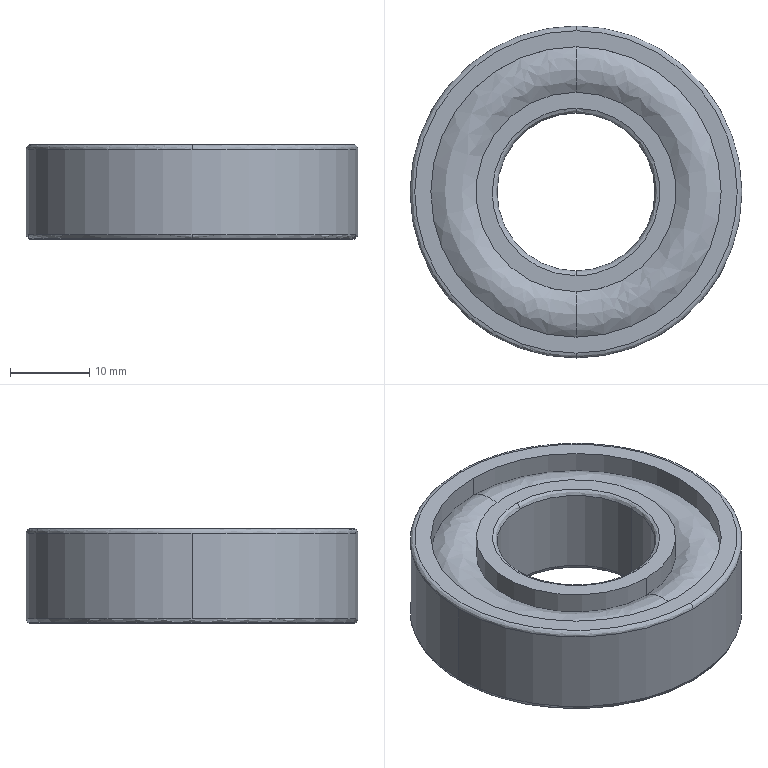Part | SolidWorks | features BaseBody 1 | 1 solid | 34 faces | box 42 x 42 x 12 mm | volume 10656 mm3 | spline 18 | cylinder 12 | plane 4 | commonest cylinder face diameters 25.25 x4 36.75 x4 20 x2 42 x2